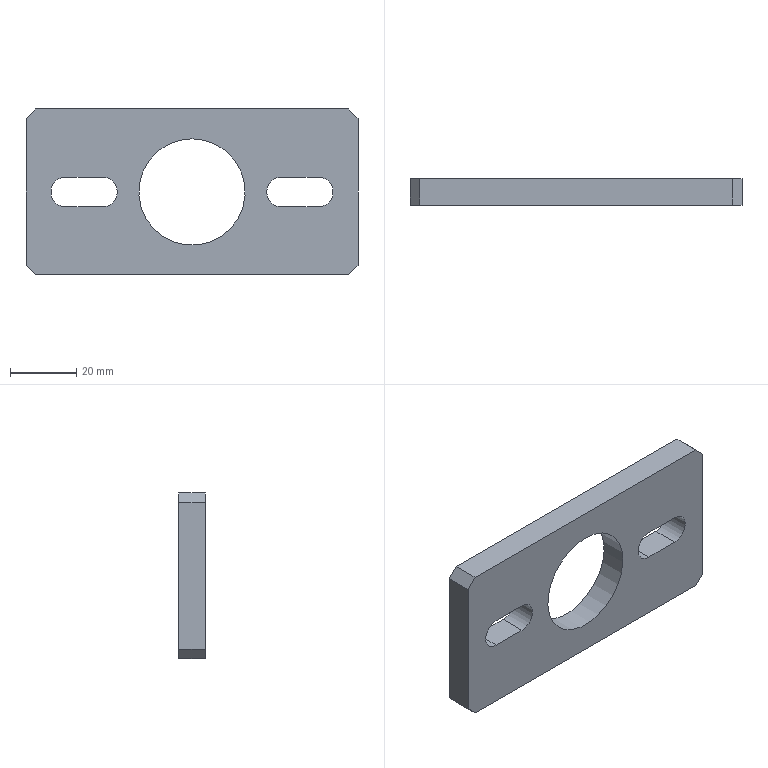Part | STEP file | PN_0067 304 guardrail mounting plate 100X50X8_Default<As Machined> | 1 solid | 19 faces | box 100 x 8 x 50 mm | volume 30820 mm3 | plane 14 | cylinder 5 | commonest cylinder face diameters 9 x4 32 x1